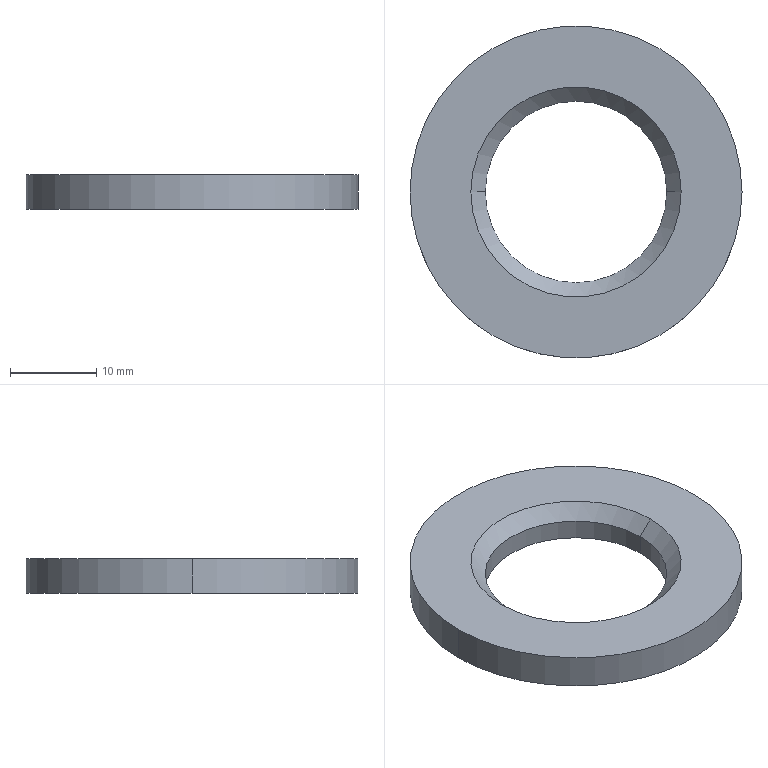Part | SolidWorks | 1 solid | 8 faces | box 38.4 x 38.4 x 4 mm | volume 3151 mm3 | cylinder 4 | cone 2 | plane 2 | commonest cylinder face diameters 21 x2 38.4 x2
STEP:
#1=CARTESIAN_POINT('',(10.5,0.,2.34));
#2=VERTEX_POINT('',#1);
#3=CARTESIAN_POINT('',(-10.5,0.,2.34));
#4=VERTEX_POINT('',#3);
#5=CARTESIAN_POINT('',(0.,0.,2.34));
#6=DIRECTION('',(0.,0.,-1.));
#7=DIRECTION('',(1.,0.,0.));
#8=AXIS2_PLACEMENT_3D('',#5,#6,#7);
#9=CIRCLE('',#8,10.5);
#10=EDGE_CURVE('',#2,#4,#9,.T.);
#11=ORIENTED_EDGE('',*,*,#10,.T.);
#12=CARTESIAN_POINT('',(-12.16,0.,4.));
#13=VERTEX_POINT('',#12);
#14=CARTESIAN_POINT('',(-12.16,0.,4.));
#15=DIRECTION('',(-0.7071,0.,0.7071));
#16=VECTOR('',#15,1000.);
#17=LINE('',#14,#16);
#18=EDGE_CURVE('',#4,#13,#17,.T.);
#19=ORIENTED_EDGE('',*,*,#18,.T.);
#20=CARTESIAN_POINT('',(12.16,0.,4.));
#21=VERTEX_POINT('',#20);
#22=CARTESIAN_POINT('',(0.,0.,4.));
#23=DIRECTION('',(0.,0.,1.));
#24=DIRECTION('',(1.,0.,0.));
#25=AXIS2_PLACEMENT_3D('',#22,#23,#24);
#26=CIRCLE('',#25,12.16);
#27=EDGE_CURVE('',#13,#21,#26,.T.);
#28=ORIENTED_EDGE('',*,*,#27,.T.);
#29=CARTESIAN_POINT('',(12.16,0.,4.));
#30=DIRECTION('',(0.7071,0.,0.7071));
#31=VECTOR('',#30,1000.);
#32=LINE('',#29,#31);
#33=EDGE_CURVE('',#2,#21,#32,.T.);
#34=ORIENTED_EDGE('',*,*,#33,.F.);
#35=EDGE_LOOP('',(#11,#19,#28,#34));
#36=FACE_OUTER_BOUND('',#35,.T.);
#37=CARTESIAN_POINT('',(0.,0.,4.));
#38=DIRECTION('',(0.,0.,1.));
#39=DIRECTION('',(1.,0.,0.));
#40=AXIS2_PLACEMENT_3D('',#37,#38,#39);
#41=CONICAL_SURFACE('',#40,12.16,0.7854);
#42=ADVANCED_FACE('',(#36),#41,.F.);
#43=ORIENTED_EDGE('',*,*,#10,.F.);
#44=CARTESIAN_POINT('',(10.5,0.,0.));
#45=VERTEX_POINT('',#44);
#46=CARTESIAN_POINT('',(10.5,0.,4.));
#47=DIRECTION('',(0.,0.,-1.));
#48=VECTOR('',#47,1000.);
#49=LINE('',#46,#48);
#50=EDGE_CURVE('',#2,#45,#49,.T.);
#51=ORIENTED_EDGE('',*,*,#50,.T.);
#52=CARTESIAN_POINT('',(-10.5,0.,0.));
#53=VERTEX_POINT('',#52);
#54=CARTESIAN_POINT('',(0.,0.,0.));
#55=DIRECTION('',(0.,0.,1.));
#56=DIRECTION('',(1.,0.,0.));
#57=AXIS2_PLACEMENT_3D('',#54,#55,#56);
#58=CIRCLE('',#57,10.5);
#59=EDGE_CURVE('',#53,#45,#58,.T.);
#60=ORIENTED_EDGE('',*,*,#59,.F.);
#61=CARTESIAN_POINT('',(-10.5,0.,4.));
#62=DIRECTION('',(0.,0.,-1.));
#63=VECTOR('',#62,1000.);
#64=LINE('',#61,#63);
#65=EDGE_CURVE('',#4,#53,#64,.T.);
#66=ORIENTED_EDGE('',*,*,#65,.F.);
#67=EDGE_LOOP('',(#43,#51,#60,#66));
#68=FACE_OUTER_BOUND('',#67,.T.);
#69=CARTESIAN_POINT('',(0.,0.,4.));
#70=DIRECTION('',(0.,0.,-1.));
#71=DIRECTION('',(-1.,0.,0.));
#72=AXIS2_PLACEMENT_3D('',#69,#70,#71);
#73=CYLINDRICAL_SURFACE('',#72,10.5);
#74=ADVANCED_FACE('',(#68),#73,.F.);
#75=CARTESIAN_POINT('',(19.2,0.,4.));
#76=VERTEX_POINT('',#75);
#77=CARTESIAN_POINT('',(-19.2,0.,4.));
#78=VERTEX_POINT('',#77);
#79=CARTESIAN_POINT('',(0.,0.,4.));
#80=DIRECTION('',(0.,0.,1.));
#81=DIRECTION('',(1.,0.,0.));
#82=AXIS2_PLACEMENT_3D('',#79,#80,#81);
#83=CIRCLE('',#82,19.2);
#84=EDGE_CURVE('',#76,#78,#83,.T.);
#85=ORIENTED_EDGE('',*,*,#84,.F.);
#86=CARTESIAN_POINT('',(19.2,0.,0.));
#87=VERTEX_POINT('',#86);
#88=CARTESIAN_POINT('',(19.2,0.,4.));
#89=DIRECTION('',(0.,0.,-1.));
#90=VECTOR('',#89,1000.);
#91=LINE('',#88,#90);
#92=EDGE_CURVE('',#76,#87,#91,.T.);
#93=ORIENTED_EDGE('',*,*,#92,.T.);
#94=CARTESIAN_POINT('',(-19.2,0.,0.));
#95=VERTEX_POINT('',#94);
#96=CARTESIAN_POINT('',(0.,0.,0.));
#97=DIRECTION('',(0.,0.,1.));
#98=DIRECTION('',(1.,0.,0.));
#99=AXIS2_PLACEMENT_3D('',#96,#97,#98);
#100=CIRCLE('',#99,19.2);
#101=EDGE_CURVE('',#87,#95,#100,.T.);
#102=ORIENTED_EDGE('',*,*,#101,.T.);
#103=CARTESIAN_POINT('',(-19.2,0.,4.));
#104=DIRECTION('',(0.,0.,-1.));
#105=VECTOR('',#104,1000.);
#106=LINE('',#103,#105);
#107=EDGE_CURVE('',#78,#95,#106,.T.);
#108=ORIENTED_EDGE('',*,*,#107,.F.);
#109=EDGE_LOOP('',(#85,#93,#102,#108));
#110=FACE_OUTER_BOUND('',#109,.T.);
#111=CARTESIAN_POINT('',(0.,0.,4.));
#112=DIRECTION('',(0.,0.,-1.));
#113=DIRECTION('',(-1.,0.,0.));
#114=AXIS2_PLACEMENT_3D('',#111,#112,#113);
#115=CYLINDRICAL_SURFACE('',#114,19.2);
#116=ADVANCED_FACE('',(#110),#115,.T.);
#117=CARTESIAN_POINT('',(0.,0.,4.));
#118=DIRECTION('',(0.,0.,1.));
#119=DIRECTION('',(1.,0.,0.));
#120=AXIS2_PLACEMENT_3D('',#117,#118,#119);
#121=CIRCLE('',#120,12.16);
#122=EDGE_CURVE('',#21,#13,#121,.T.);
#123=ORIENTED_EDGE('',*,*,#122,.F.);
#124=ORIENTED_EDGE('',*,*,#27,.F.);
#125=EDGE_LOOP('',(#123,#124));
#126=FACE_BOUND('',#125,.T.);
#127=CARTESIAN_POINT('',(0.,0.,4.));
#128=DIRECTION('',(0.,0.,1.));
#129=DIRECTION('',(1.,0.,0.));
#130=AXIS2_PLACEMENT_3D('',#127,#128,#129);
#131=CIRCLE('',#130,19.2);
#132=EDGE_CURVE('',#78,#76,#131,.T.);
#133=ORIENTED_EDGE('',*,*,#132,.T.);
#134=ORIENTED_EDGE('',*,*,#84,.T.);
#135=EDGE_LOOP('',(#133,#134));
#136=FACE_OUTER_BOUND('',#135,.T.);
#137=CARTESIAN_POINT('',(0.,0.,4.));
#138=DIRECTION('',(0.,0.,1.));
#139=DIRECTION('',(1.,0.,0.));
#140=AXIS2_PLACEMENT_3D('',#137,#138,#139);
#141=PLANE('',#140);
#142=ADVANCED_FACE('',(#126,#136),#141,.T.);
#143=CARTESIAN_POINT('',(0.,0.,0.));
#144=DIRECTION('',(0.,0.,1.));
#145=DIRECTION('',(1.,0.,0.));
#146=AXIS2_PLACEMENT_3D('',#143,#144,#145);
#147=CIRCLE('',#146,19.2);
#148=EDGE_CURVE('',#95,#87,#147,.T.);
#149=ORIENTED_EDGE('',*,*,#148,.F.);
#150=ORIENTED_EDGE('',*,*,#101,.F.);
#151=EDGE_LOOP('',(#149,#150));
#152=FACE_OUTER_BOUND('',#151,.T.);
#153=ORIENTED_EDGE('',*,*,#59,.T.);
#154=CARTESIAN_POINT('',(0.,0.,0.));
#155=DIRECTION('',(0.,0.,1.));
#156=DIRECTION('',(1.,0.,0.));
#157=AXIS2_PLACEMENT_3D('',#154,#155,#156);
#158=CIRCLE('',#157,10.5);
#159=EDGE_CURVE('',#45,#53,#158,.T.);
#160=ORIENTED_EDGE('',*,*,#159,.T.);
#161=EDGE_LOOP('',(#153,#160));
#162=FACE_BOUND('',#161,.T.);
#163=CARTESIAN_POINT('',(0.,0.,0.));
#164=DIRECTION('',(0.,0.,1.));
#165=DIRECTION('',(1.,0.,0.));
#166=AXIS2_PLACEMENT_3D('',#163,#164,#165);
#167=PLANE('',#166);
#168=ADVANCED_FACE('',(#152,#162),#167,.F.);
#169=ORIENTED_EDGE('',*,*,#92,.F.);
#170=ORIENTED_EDGE('',*,*,#132,.F.);
#171=ORIENTED_EDGE('',*,*,#107,.T.);
#172=ORIENTED_EDGE('',*,*,#148,.T.);
#173=EDGE_LOOP('',(#169,#170,#171,#172));
#174=FACE_OUTER_BOUND('',#173,.T.);
#175=CARTESIAN_POINT('',(0.,0.,4.));
#176=DIRECTION('',(0.,0.,-1.));
#177=DIRECTION('',(-1.,0.,0.));
#178=AXIS2_PLACEMENT_3D('',#175,#176,#177);
#179=CYLINDRICAL_SURFACE('',#178,19.2);
#180=ADVANCED_FACE('',(#174),#179,.T.);
#181=ORIENTED_EDGE('',*,*,#50,.F.);
#182=CARTESIAN_POINT('',(0.,0.,2.34));
#183=DIRECTION('',(0.,0.,-1.));
#184=DIRECTION('',(1.,0.,0.));
#185=AXIS2_PLACEMENT_3D('',#182,#183,#184);
#186=CIRCLE('',#185,10.5);
#187=EDGE_CURVE('',#4,#2,#186,.T.);
#188=ORIENTED_EDGE('',*,*,#187,.F.);
#189=ORIENTED_EDGE('',*,*,#65,.T.);
#190=ORIENTED_EDGE('',*,*,#159,.F.);
#191=EDGE_LOOP('',(#181,#188,#189,#190));
#192=FACE_OUTER_BOUND('',#191,.T.);
#193=CARTESIAN_POINT('',(0.,0.,4.));
#194=DIRECTION('',(0.,0.,-1.));
#195=DIRECTION('',(-1.,0.,0.));
#196=AXIS2_PLACEMENT_3D('',#193,#194,#195);
#197=CYLINDRICAL_SURFACE('',#196,10.5);
#198=ADVANCED_FACE('',(#192),#197,.F.);
#199=ORIENTED_EDGE('',*,*,#18,.F.);
#200=ORIENTED_EDGE('',*,*,#187,.T.);
#201=ORIENTED_EDGE('',*,*,#33,.T.);
#202=ORIENTED_EDGE('',*,*,#122,.T.);
#203=EDGE_LOOP('',(#199,#200,#201,#202));
#204=FACE_OUTER_BOUND('',#203,.T.);
#205=CARTESIAN_POINT('',(0.,0.,4.));
#206=DIRECTION('',(0.,0.,1.));
#207=DIRECTION('',(1.,0.,0.));
#208=AXIS2_PLACEMENT_3D('',#205,#206,#207);
#209=CONICAL_SURFACE('',#208,12.16,0.7854);
#210=ADVANCED_FACE('',(#204),#209,.F.);
#211=CLOSED_SHELL('',(#42,#74,#116,#142,#168,#180,#198,#210));
#212=MANIFOLD_SOLID_BREP('',#211);
#213=CARTESIAN_POINT('',(0.,0.,0.));
#214=DIRECTION('',(0.,0.,1.));
#215=DIRECTION('',(1.,0.,0.));
#216=AXIS2_PLACEMENT_3D('',#213,#214,#215);
#217=(LENGTH_UNIT()NAMED_UNIT(*)SI_UNIT(.MILLI.,.METRE.));
#218=UNCERTAINTY_MEASURE_WITH_UNIT(LENGTH_MEASURE(0.00001),#217,'','');
#219=(NAMED_UNIT(*)PLANE_ANGLE_UNIT()SI_UNIT($,.RADIAN.));
#220=(NAMED_UNIT(*)SI_UNIT($,.STERADIAN.)SOLID_ANGLE_UNIT());
#221=(GEOMETRIC_REPRESENTATION_CONTEXT(3)GLOBAL_UNCERTAINTY_ASSIGNED_CONTEXT((#218))GLOBAL_UNIT_ASSIGNED_CONTEXT((#217,#219,#220))REPRESENTATION_CONTEXT('',''));
#222=ADVANCED_BREP_SHAPE_REPRESENTATION('',(#212,#216),#221);